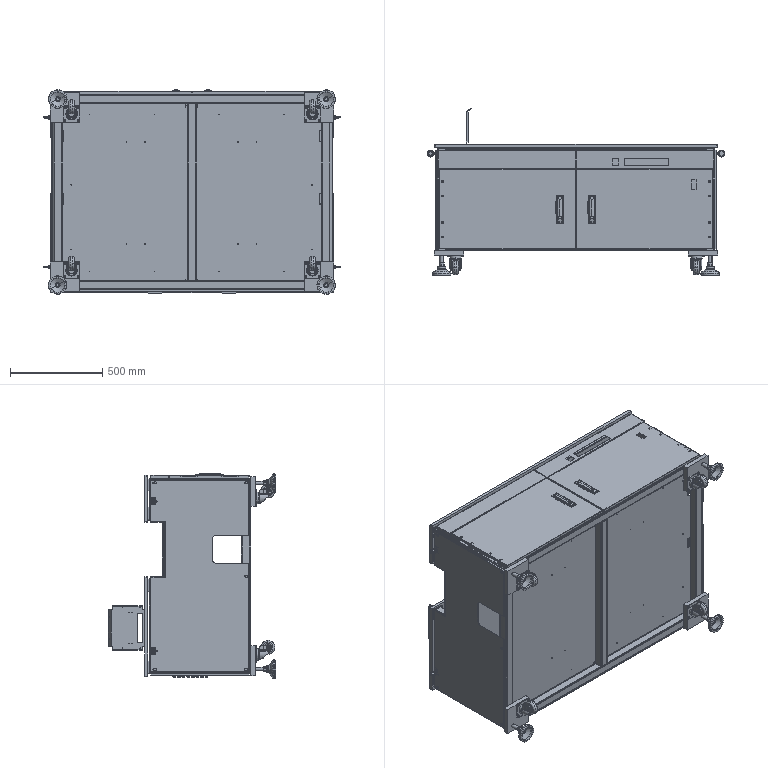Part | NX | features BREP 69 | 92 solids | 3542 faces | volume 39960474 mm3 | plane 1683 | cylinder 1497 | cone 140 | torus 120 | spline 76 | sphere 26 | commonest cylinder face diameters 3.3 x200 10 x131 8 x104 5 x100 6 x76 12 x76